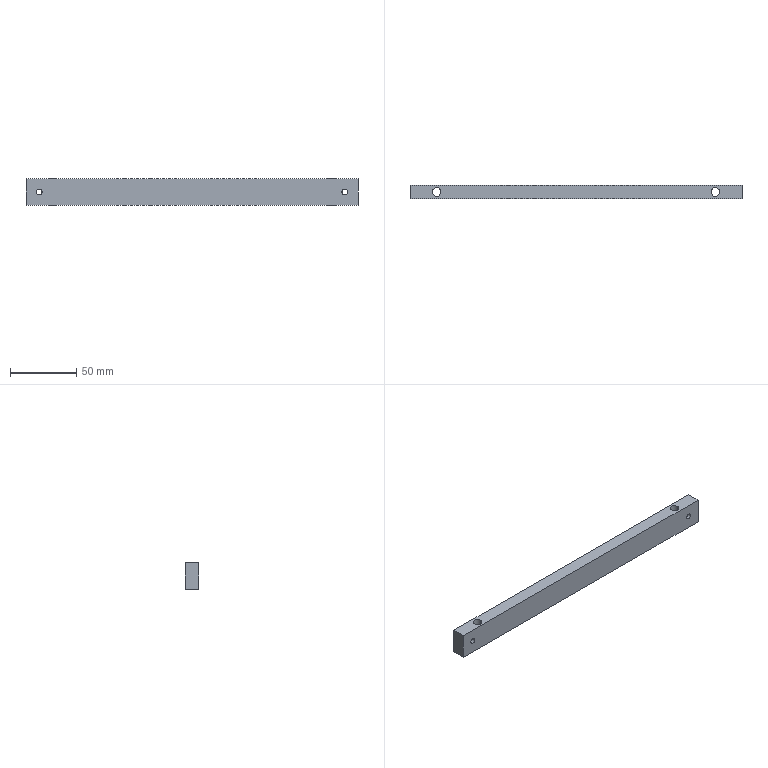Part | STEP file | Insert strip | 1 solid | 14 faces | box 250 x 10 x 20 mm | volume 48396 mm3 | cylinder 8 | plane 6 | commonest cylinder face diameters 4.2 x4 6.5 x4
STEP:
#1=CARTESIAN_POINT('',(115.,-5.,7.9));
#2=VERTEX_POINT('',#1);
#3=CARTESIAN_POINT('',(115.,-5.,12.1));
#4=VERTEX_POINT('',#3);
#5=CARTESIAN_POINT('',(115.,-5.,10.));
#6=DIRECTION('',(0.,1.,0.));
#7=DIRECTION('',(0.,0.,1.));
#8=AXIS2_PLACEMENT_3D('',#5,#6,#7);
#9=CIRCLE('',#8,2.1);
#10=EDGE_CURVE('',#2,#4,#9,.T.);
#11=ORIENTED_EDGE('',*,*,#10,.F.);
#12=CARTESIAN_POINT('',(115.,5.,7.9));
#13=VERTEX_POINT('',#12);
#14=CARTESIAN_POINT('',(115.,5.,7.9));
#15=DIRECTION('',(0.,1.,0.));
#16=VECTOR('',#15,1000.);
#17=LINE('',#14,#16);
#18=EDGE_CURVE('',#2,#13,#17,.T.);
#19=ORIENTED_EDGE('',*,*,#18,.T.);
#20=CARTESIAN_POINT('',(115.,5.,12.1));
#21=VERTEX_POINT('',#20);
#22=CARTESIAN_POINT('',(115.,5.,10.));
#23=DIRECTION('',(0.,1.,0.));
#24=DIRECTION('',(0.,0.,1.));
#25=AXIS2_PLACEMENT_3D('',#22,#23,#24);
#26=CIRCLE('',#25,2.1);
#27=EDGE_CURVE('',#13,#21,#26,.T.);
#28=ORIENTED_EDGE('',*,*,#27,.T.);
#29=CARTESIAN_POINT('',(115.,5.,12.1));
#30=DIRECTION('',(0.,1.,0.));
#31=VECTOR('',#30,1000.);
#32=LINE('',#29,#31);
#33=EDGE_CURVE('',#4,#21,#32,.T.);
#34=ORIENTED_EDGE('',*,*,#33,.F.);
#35=EDGE_LOOP('',(#11,#19,#28,#34));
#36=FACE_OUTER_BOUND('',#35,.T.);
#37=CARTESIAN_POINT('',(115.,5.,10.));
#38=DIRECTION('',(0.,1.,0.));
#39=DIRECTION('',(0.,0.,1.));
#40=AXIS2_PLACEMENT_3D('',#37,#38,#39);
#41=CYLINDRICAL_SURFACE('',#40,2.1);
#42=ADVANCED_FACE('',(#36),#41,.F.);
#43=CARTESIAN_POINT('',(-115.,-5.,7.9));
#44=VERTEX_POINT('',#43);
#45=CARTESIAN_POINT('',(-115.,-5.,12.1));
#46=VERTEX_POINT('',#45);
#47=CARTESIAN_POINT('',(-115.,-5.,10.));
#48=DIRECTION('',(0.,1.,0.));
#49=DIRECTION('',(0.,0.,1.));
#50=AXIS2_PLACEMENT_3D('',#47,#48,#49);
#51=CIRCLE('',#50,2.1);
#52=EDGE_CURVE('',#44,#46,#51,.T.);
#53=ORIENTED_EDGE('',*,*,#52,.F.);
#54=CARTESIAN_POINT('',(-115.,5.,7.9));
#55=VERTEX_POINT('',#54);
#56=CARTESIAN_POINT('',(-115.,5.,7.9));
#57=DIRECTION('',(0.,1.,0.));
#58=VECTOR('',#57,1000.);
#59=LINE('',#56,#58);
#60=EDGE_CURVE('',#44,#55,#59,.T.);
#61=ORIENTED_EDGE('',*,*,#60,.T.);
#62=CARTESIAN_POINT('',(-115.,5.,12.1));
#63=VERTEX_POINT('',#62);
#64=CARTESIAN_POINT('',(-115.,5.,10.));
#65=DIRECTION('',(0.,1.,0.));
#66=DIRECTION('',(0.,0.,1.));
#67=AXIS2_PLACEMENT_3D('',#64,#65,#66);
#68=CIRCLE('',#67,2.1);
#69=EDGE_CURVE('',#55,#63,#68,.T.);
#70=ORIENTED_EDGE('',*,*,#69,.T.);
#71=CARTESIAN_POINT('',(-115.,5.,12.1));
#72=DIRECTION('',(0.,1.,0.));
#73=VECTOR('',#72,1000.);
#74=LINE('',#71,#73);
#75=EDGE_CURVE('',#46,#63,#74,.T.);
#76=ORIENTED_EDGE('',*,*,#75,.F.);
#77=EDGE_LOOP('',(#53,#61,#70,#76));
#78=FACE_OUTER_BOUND('',#77,.T.);
#79=CARTESIAN_POINT('',(-115.,5.,10.));
#80=DIRECTION('',(0.,1.,0.));
#81=DIRECTION('',(0.,0.,1.));
#82=AXIS2_PLACEMENT_3D('',#79,#80,#81);
#83=CYLINDRICAL_SURFACE('',#82,2.1);
#84=ADVANCED_FACE('',(#78),#83,.F.);
#85=CARTESIAN_POINT('',(-108.25,0.,0.));
#86=VERTEX_POINT('',#85);
#87=CARTESIAN_POINT('',(-101.75,0.,0.));
#88=VERTEX_POINT('',#87);
#89=CARTESIAN_POINT('',(-105.,0.,0.));
#90=DIRECTION('',(0.,0.,1.));
#91=DIRECTION('',(1.,0.,0.));
#92=AXIS2_PLACEMENT_3D('',#89,#90,#91);
#93=CIRCLE('',#92,3.25);
#94=EDGE_CURVE('',#86,#88,#93,.T.);
#95=ORIENTED_EDGE('',*,*,#94,.F.);
#96=CARTESIAN_POINT('',(-108.25,0.,20.));
#97=VERTEX_POINT('',#96);
#98=CARTESIAN_POINT('',(-108.25,0.,20.));
#99=DIRECTION('',(0.,0.,1.));
#100=VECTOR('',#99,1000.);
#101=LINE('',#98,#100);
#102=EDGE_CURVE('',#86,#97,#101,.T.);
#103=ORIENTED_EDGE('',*,*,#102,.T.);
#104=CARTESIAN_POINT('',(-101.75,0.,20.));
#105=VERTEX_POINT('',#104);
#106=CARTESIAN_POINT('',(-105.,0.,20.));
#107=DIRECTION('',(0.,0.,1.));
#108=DIRECTION('',(1.,0.,0.));
#109=AXIS2_PLACEMENT_3D('',#106,#107,#108);
#110=CIRCLE('',#109,3.25);
#111=EDGE_CURVE('',#97,#105,#110,.T.);
#112=ORIENTED_EDGE('',*,*,#111,.T.);
#113=CARTESIAN_POINT('',(-101.75,0.,20.));
#114=DIRECTION('',(0.,0.,1.));
#115=VECTOR('',#114,1000.);
#116=LINE('',#113,#115);
#117=EDGE_CURVE('',#88,#105,#116,.T.);
#118=ORIENTED_EDGE('',*,*,#117,.F.);
#119=EDGE_LOOP('',(#95,#103,#112,#118));
#120=FACE_OUTER_BOUND('',#119,.T.);
#121=CARTESIAN_POINT('',(-105.,0.,20.));
#122=DIRECTION('',(0.,0.,1.));
#123=DIRECTION('',(1.,0.,0.));
#124=AXIS2_PLACEMENT_3D('',#121,#122,#123);
#125=CYLINDRICAL_SURFACE('',#124,3.25);
#126=ADVANCED_FACE('',(#120),#125,.F.);
#127=CARTESIAN_POINT('',(101.75,0.,0.));
#128=VERTEX_POINT('',#127);
#129=CARTESIAN_POINT('',(108.25,0.,0.));
#130=VERTEX_POINT('',#129);
#131=CARTESIAN_POINT('',(105.,0.,0.));
#132=DIRECTION('',(0.,0.,1.));
#133=DIRECTION('',(1.,0.,0.));
#134=AXIS2_PLACEMENT_3D('',#131,#132,#133);
#135=CIRCLE('',#134,3.25);
#136=EDGE_CURVE('',#128,#130,#135,.T.);
#137=ORIENTED_EDGE('',*,*,#136,.F.);
#138=CARTESIAN_POINT('',(101.75,0.,20.));
#139=VERTEX_POINT('',#138);
#140=CARTESIAN_POINT('',(101.75,0.,20.));
#141=DIRECTION('',(0.,0.,1.));
#142=VECTOR('',#141,1000.);
#143=LINE('',#140,#142);
#144=EDGE_CURVE('',#128,#139,#143,.T.);
#145=ORIENTED_EDGE('',*,*,#144,.T.);
#146=CARTESIAN_POINT('',(108.25,0.,20.));
#147=VERTEX_POINT('',#146);
#148=CARTESIAN_POINT('',(105.,0.,20.));
#149=DIRECTION('',(0.,0.,1.));
#150=DIRECTION('',(1.,0.,0.));
#151=AXIS2_PLACEMENT_3D('',#148,#149,#150);
#152=CIRCLE('',#151,3.25);
#153=EDGE_CURVE('',#139,#147,#152,.T.);
#154=ORIENTED_EDGE('',*,*,#153,.T.);
#155=CARTESIAN_POINT('',(108.25,0.,20.));
#156=DIRECTION('',(0.,0.,1.));
#157=VECTOR('',#156,1000.);
#158=LINE('',#155,#157);
#159=EDGE_CURVE('',#130,#147,#158,.T.);
#160=ORIENTED_EDGE('',*,*,#159,.F.);
#161=EDGE_LOOP('',(#137,#145,#154,#160));
#162=FACE_OUTER_BOUND('',#161,.T.);
#163=CARTESIAN_POINT('',(105.,0.,20.));
#164=DIRECTION('',(0.,0.,1.));
#165=DIRECTION('',(1.,0.,0.));
#166=AXIS2_PLACEMENT_3D('',#163,#164,#165);
#167=CYLINDRICAL_SURFACE('',#166,3.25);
#168=ADVANCED_FACE('',(#162),#167,.F.);
#169=CARTESIAN_POINT('',(125.,-5.,0.));
#170=VERTEX_POINT('',#169);
#171=CARTESIAN_POINT('',(125.,5.,0.));
#172=VERTEX_POINT('',#171);
#173=CARTESIAN_POINT('',(125.,-5.,0.));
#174=DIRECTION('',(0.,1.,0.));
#175=VECTOR('',#174,1000.);
#176=LINE('',#173,#175);
#177=EDGE_CURVE('',#170,#172,#176,.T.);
#178=ORIENTED_EDGE('',*,*,#177,.T.);
#179=CARTESIAN_POINT('',(125.,5.,20.));
#180=VERTEX_POINT('',#179);
#181=CARTESIAN_POINT('',(125.,5.,20.));
#182=DIRECTION('',(0.,0.,-1.));
#183=VECTOR('',#182,1000.);
#184=LINE('',#181,#183);
#185=EDGE_CURVE('',#180,#172,#184,.T.);
#186=ORIENTED_EDGE('',*,*,#185,.F.);
#187=CARTESIAN_POINT('',(125.,-5.,20.));
#188=VERTEX_POINT('',#187);
#189=CARTESIAN_POINT('',(125.,-5.,20.));
#190=DIRECTION('',(0.,1.,0.));
#191=VECTOR('',#190,1000.);
#192=LINE('',#189,#191);
#193=EDGE_CURVE('',#188,#180,#192,.T.);
#194=ORIENTED_EDGE('',*,*,#193,.F.);
#195=CARTESIAN_POINT('',(125.,-5.,20.));
#196=DIRECTION('',(0.,0.,-1.));
#197=VECTOR('',#196,1000.);
#198=LINE('',#195,#197);
#199=EDGE_CURVE('',#188,#170,#198,.T.);
#200=ORIENTED_EDGE('',*,*,#199,.T.);
#201=EDGE_LOOP('',(#178,#186,#194,#200));
#202=FACE_OUTER_BOUND('',#201,.T.);
#203=CARTESIAN_POINT('',(125.,-5.,20.));
#204=DIRECTION('',(-1.,0.,0.));
#205=DIRECTION('',(0.,0.,1.));
#206=AXIS2_PLACEMENT_3D('',#203,#204,#205);
#207=PLANE('',#206);
#208=ADVANCED_FACE('',(#202),#207,.F.);
#209=CARTESIAN_POINT('',(115.,5.,10.));
#210=DIRECTION('',(0.,1.,0.));
#211=DIRECTION('',(0.,0.,1.));
#212=AXIS2_PLACEMENT_3D('',#209,#210,#211);
#213=CIRCLE('',#212,2.1);
#214=EDGE_CURVE('',#21,#13,#213,.T.);
#215=ORIENTED_EDGE('',*,*,#214,.F.);
#216=ORIENTED_EDGE('',*,*,#27,.F.);
#217=EDGE_LOOP('',(#215,#216));
#218=FACE_BOUND('',#217,.T.);
#219=CARTESIAN_POINT('',(-115.,5.,10.));
#220=DIRECTION('',(0.,1.,0.));
#221=DIRECTION('',(0.,0.,1.));
#222=AXIS2_PLACEMENT_3D('',#219,#220,#221);
#223=CIRCLE('',#222,2.1);
#224=EDGE_CURVE('',#63,#55,#223,.T.);
#225=ORIENTED_EDGE('',*,*,#224,.F.);
#226=ORIENTED_EDGE('',*,*,#69,.F.);
#227=EDGE_LOOP('',(#225,#226));
#228=FACE_BOUND('',#227,.T.);
#229=CARTESIAN_POINT('',(-125.,5.,0.));
#230=VERTEX_POINT('',#229);
#231=CARTESIAN_POINT('',(-125.,5.,0.));
#232=DIRECTION('',(-1.,0.,0.));
#233=VECTOR('',#232,1000.);
#234=LINE('',#231,#233);
#235=EDGE_CURVE('',#172,#230,#234,.T.);
#236=ORIENTED_EDGE('',*,*,#235,.T.);
#237=CARTESIAN_POINT('',(-125.,5.,20.));
#238=VERTEX_POINT('',#237);
#239=CARTESIAN_POINT('',(-125.,5.,20.));
#240=DIRECTION('',(0.,0.,-1.));
#241=VECTOR('',#240,1000.);
#242=LINE('',#239,#241);
#243=EDGE_CURVE('',#238,#230,#242,.T.);
#244=ORIENTED_EDGE('',*,*,#243,.F.);
#245=CARTESIAN_POINT('',(-125.,5.,20.));
#246=DIRECTION('',(-1.,0.,0.));
#247=VECTOR('',#246,1000.);
#248=LINE('',#245,#247);
#249=EDGE_CURVE('',#180,#238,#248,.T.);
#250=ORIENTED_EDGE('',*,*,#249,.F.);
#251=ORIENTED_EDGE('',*,*,#185,.T.);
#252=EDGE_LOOP('',(#236,#244,#250,#251));
#253=FACE_OUTER_BOUND('',#252,.T.);
#254=CARTESIAN_POINT('',(-125.,5.,20.));
#255=DIRECTION('',(0.,-1.,0.));
#256=DIRECTION('',(0.,0.,-1.));
#257=AXIS2_PLACEMENT_3D('',#254,#255,#256);
#258=PLANE('',#257);
#259=ADVANCED_FACE('',(#218,#228,#253),#258,.F.);
#260=CARTESIAN_POINT('',(-125.,-5.,0.));
#261=VERTEX_POINT('',#260);
#262=CARTESIAN_POINT('',(-125.,-5.,0.));
#263=DIRECTION('',(0.,-1.,0.));
#264=VECTOR('',#263,1000.);
#265=LINE('',#262,#264);
#266=EDGE_CURVE('',#230,#261,#265,.T.);
#267=ORIENTED_EDGE('',*,*,#266,.T.);
#268=CARTESIAN_POINT('',(-125.,-5.,20.));
#269=VERTEX_POINT('',#268);
#270=CARTESIAN_POINT('',(-125.,-5.,20.));
#271=DIRECTION('',(0.,0.,-1.));
#272=VECTOR('',#271,1000.);
#273=LINE('',#270,#272);
#274=EDGE_CURVE('',#269,#261,#273,.T.);
#275=ORIENTED_EDGE('',*,*,#274,.F.);
#276=CARTESIAN_POINT('',(-125.,-5.,20.));
#277=DIRECTION('',(0.,-1.,0.));
#278=VECTOR('',#277,1000.);
#279=LINE('',#276,#278);
#280=EDGE_CURVE('',#238,#269,#279,.T.);
#281=ORIENTED_EDGE('',*,*,#280,.F.);
#282=ORIENTED_EDGE('',*,*,#243,.T.);
#283=EDGE_LOOP('',(#267,#275,#281,#282));
#284=FACE_OUTER_BOUND('',#283,.T.);
#285=CARTESIAN_POINT('',(-125.,-5.,20.));
#286=DIRECTION('',(1.,0.,0.));
#287=DIRECTION('',(0.,0.,-1.));
#288=AXIS2_PLACEMENT_3D('',#285,#286,#287);
#289=PLANE('',#288);
#290=ADVANCED_FACE('',(#284),#289,.F.);
#291=CARTESIAN_POINT('',(115.,-5.,10.));
#292=DIRECTION('',(0.,1.,0.));
#293=DIRECTION('',(0.,0.,1.));
#294=AXIS2_PLACEMENT_3D('',#291,#292,#293);
#295=CIRCLE('',#294,2.1);
#296=EDGE_CURVE('',#4,#2,#295,.T.);
#297=ORIENTED_EDGE('',*,*,#296,.T.);
#298=ORIENTED_EDGE('',*,*,#10,.T.);
#299=EDGE_LOOP('',(#297,#298));
#300=FACE_BOUND('',#299,.T.);
#301=CARTESIAN_POINT('',(-115.,-5.,10.));
#302=DIRECTION('',(0.,1.,0.));
#303=DIRECTION('',(0.,0.,1.));
#304=AXIS2_PLACEMENT_3D('',#301,#302,#303);
#305=CIRCLE('',#304,2.1);
#306=EDGE_CURVE('',#46,#44,#305,.T.);
#307=ORIENTED_EDGE('',*,*,#306,.T.);
#308=ORIENTED_EDGE('',*,*,#52,.T.);
#309=EDGE_LOOP('',(#307,#308));
#310=FACE_BOUND('',#309,.T.);
#311=CARTESIAN_POINT('',(-125.,-5.,0.));
#312=DIRECTION('',(1.,0.,0.));
#313=VECTOR('',#312,1000.);
#314=LINE('',#311,#313);
#315=EDGE_CURVE('',#261,#170,#314,.T.);
#316=ORIENTED_EDGE('',*,*,#315,.T.);
#317=ORIENTED_EDGE('',*,*,#199,.F.);
#318=CARTESIAN_POINT('',(-125.,-5.,20.));
#319=DIRECTION('',(1.,0.,0.));
#320=VECTOR('',#319,1000.);
#321=LINE('',#318,#320);
#322=EDGE_CURVE('',#269,#188,#321,.T.);
#323=ORIENTED_EDGE('',*,*,#322,.F.);
#324=ORIENTED_EDGE('',*,*,#274,.T.);
#325=EDGE_LOOP('',(#316,#317,#323,#324));
#326=FACE_OUTER_BOUND('',#325,.T.);
#327=CARTESIAN_POINT('',(-125.,-5.,20.));
#328=DIRECTION('',(0.,1.,0.));
#329=DIRECTION('',(0.,0.,1.));
#330=AXIS2_PLACEMENT_3D('',#327,#328,#329);
#331=PLANE('',#330);
#332=ADVANCED_FACE('',(#300,#310,#326),#331,.F.);
#333=CARTESIAN_POINT('',(-105.,0.,20.));
#334=DIRECTION('',(0.,0.,1.));
#335=DIRECTION('',(1.,0.,0.));
#336=AXIS2_PLACEMENT_3D('',#333,#334,#335);
#337=CIRCLE('',#336,3.25);
#338=EDGE_CURVE('',#105,#97,#337,.T.);
#339=ORIENTED_EDGE('',*,*,#338,.F.);
#340=ORIENTED_EDGE('',*,*,#111,.F.);
#341=EDGE_LOOP('',(#339,#340));
#342=FACE_BOUND('',#341,.T.);
#343=CARTESIAN_POINT('',(105.,0.,20.));
#344=DIRECTION('',(0.,0.,1.));
#345=DIRECTION('',(1.,0.,0.));
#346=AXIS2_PLACEMENT_3D('',#343,#344,#345);
#347=CIRCLE('',#346,3.25);
#348=EDGE_CURVE('',#147,#139,#347,.T.);
#349=ORIENTED_EDGE('',*,*,#348,.F.);
#350=ORIENTED_EDGE('',*,*,#153,.F.);
#351=EDGE_LOOP('',(#349,#350));
#352=FACE_BOUND('',#351,.T.);
#353=ORIENTED_EDGE('',*,*,#193,.T.);
#354=ORIENTED_EDGE('',*,*,#249,.T.);
#355=ORIENTED_EDGE('',*,*,#280,.T.);
#356=ORIENTED_EDGE('',*,*,#322,.T.);
#357=EDGE_LOOP('',(#353,#354,#355,#356));
#358=FACE_OUTER_BOUND('',#357,.T.);
#359=CARTESIAN_POINT('',(125.,5.,20.));
#360=DIRECTION('',(0.,0.,-1.));
#361=DIRECTION('',(-1.,0.,0.));
#362=AXIS2_PLACEMENT_3D('',#359,#360,#361);
#363=PLANE('',#362);
#364=ADVANCED_FACE('',(#342,#352,#358),#363,.F.);
#365=CARTESIAN_POINT('',(-105.,0.,0.));
#366=DIRECTION('',(0.,0.,1.));
#367=DIRECTION('',(1.,0.,0.));
#368=AXIS2_PLACEMENT_3D('',#365,#366,#367);
#369=CIRCLE('',#368,3.25);
#370=EDGE_CURVE('',#88,#86,#369,.T.);
#371=ORIENTED_EDGE('',*,*,#370,.T.);
#372=ORIENTED_EDGE('',*,*,#94,.T.);
#373=EDGE_LOOP('',(#371,#372));
#374=FACE_BOUND('',#373,.T.);
#375=CARTESIAN_POINT('',(105.,0.,0.));
#376=DIRECTION('',(0.,0.,1.));
#377=DIRECTION('',(1.,0.,0.));
#378=AXIS2_PLACEMENT_3D('',#375,#376,#377);
#379=CIRCLE('',#378,3.25);
#380=EDGE_CURVE('',#130,#128,#379,.T.);
#381=ORIENTED_EDGE('',*,*,#380,.T.);
#382=ORIENTED_EDGE('',*,*,#136,.T.);
#383=EDGE_LOOP('',(#381,#382));
#384=FACE_BOUND('',#383,.T.);
#385=ORIENTED_EDGE('',*,*,#177,.F.);
#386=ORIENTED_EDGE('',*,*,#315,.F.);
#387=ORIENTED_EDGE('',*,*,#266,.F.);
#388=ORIENTED_EDGE('',*,*,#235,.F.);
#389=EDGE_LOOP('',(#385,#386,#387,#388));
#390=FACE_OUTER_BOUND('',#389,.T.);
#391=CARTESIAN_POINT('',(125.,5.,0.));
#392=DIRECTION('',(0.,0.,-1.));
#393=DIRECTION('',(-1.,0.,0.));
#394=AXIS2_PLACEMENT_3D('',#391,#392,#393);
#395=PLANE('',#394);
#396=ADVANCED_FACE('',(#374,#384,#390),#395,.T.);
#397=ORIENTED_EDGE('',*,*,#144,.F.);
#398=ORIENTED_EDGE('',*,*,#380,.F.);
#399=ORIENTED_EDGE('',*,*,#159,.T.);
#400=ORIENTED_EDGE('',*,*,#348,.T.);
#401=EDGE_LOOP('',(#397,#398,#399,#400));
#402=FACE_OUTER_BOUND('',#401,.T.);
#403=CARTESIAN_POINT('',(105.,0.,20.));
#404=DIRECTION('',(0.,0.,1.));
#405=DIRECTION('',(1.,0.,0.));
#406=AXIS2_PLACEMENT_3D('',#403,#404,#405);
#407=CYLINDRICAL_SURFACE('',#406,3.25);
#408=ADVANCED_FACE('',(#402),#407,.F.);
#409=ORIENTED_EDGE('',*,*,#102,.F.);
#410=ORIENTED_EDGE('',*,*,#370,.F.);
#411=ORIENTED_EDGE('',*,*,#117,.T.);
#412=ORIENTED_EDGE('',*,*,#338,.T.);
#413=EDGE_LOOP('',(#409,#410,#411,#412));
#414=FACE_OUTER_BOUND('',#413,.T.);
#415=CARTESIAN_POINT('',(-105.,0.,20.));
#416=DIRECTION('',(0.,0.,1.));
#417=DIRECTION('',(1.,0.,0.));
#418=AXIS2_PLACEMENT_3D('',#415,#416,#417);
#419=CYLINDRICAL_SURFACE('',#418,3.25);
#420=ADVANCED_FACE('',(#414),#419,.F.);
#421=ORIENTED_EDGE('',*,*,#60,.F.);
#422=ORIENTED_EDGE('',*,*,#306,.F.);
#423=ORIENTED_EDGE('',*,*,#75,.T.);
#424=ORIENTED_EDGE('',*,*,#224,.T.);
#425=EDGE_LOOP('',(#421,#422,#423,#424));
#426=FACE_OUTER_BOUND('',#425,.T.);
#427=CARTESIAN_POINT('',(-115.,5.,10.));
#428=DIRECTION('',(0.,1.,0.));
#429=DIRECTION('',(0.,0.,1.));
#430=AXIS2_PLACEMENT_3D('',#427,#428,#429);
#431=CYLINDRICAL_SURFACE('',#430,2.1);
#432=ADVANCED_FACE('',(#426),#431,.F.);
#433=ORIENTED_EDGE('',*,*,#18,.F.);
#434=ORIENTED_EDGE('',*,*,#296,.F.);
#435=ORIENTED_EDGE('',*,*,#33,.T.);
#436=ORIENTED_EDGE('',*,*,#214,.T.);
#437=EDGE_LOOP('',(#433,#434,#435,#436));
#438=FACE_OUTER_BOUND('',#437,.T.);
#439=CARTESIAN_POINT('',(115.,5.,10.));
#440=DIRECTION('',(0.,1.,0.));
#441=DIRECTION('',(0.,0.,1.));
#442=AXIS2_PLACEMENT_3D('',#439,#440,#441);
#443=CYLINDRICAL_SURFACE('',#442,2.1);
#444=ADVANCED_FACE('',(#438),#443,.F.);
#445=CLOSED_SHELL('',(#42,#84,#126,#168,#208,#259,#290,#332,#364,#396,#408,#420,#432,#444));
#446=MANIFOLD_SOLID_BREP('',#445);
#447=CARTESIAN_POINT('',(0.,0.,0.));
#448=DIRECTION('',(0.,0.,1.));
#449=DIRECTION('',(1.,0.,0.));
#450=AXIS2_PLACEMENT_3D('',#447,#448,#449);
#451=(LENGTH_UNIT()NAMED_UNIT(*)SI_UNIT(.MILLI.,.METRE.));
#452=UNCERTAINTY_MEASURE_WITH_UNIT(LENGTH_MEASURE(0.00001),#451,'','');
#453=(NAMED_UNIT(*)PLANE_ANGLE_UNIT()SI_UNIT($,.RADIAN.));
#454=(NAMED_UNIT(*)SI_UNIT($,.STERADIAN.)SOLID_ANGLE_UNIT());
#455=(GEOMETRIC_REPRESENTATION_CONTEXT(3)GLOBAL_UNCERTAINTY_ASSIGNED_CONTEXT((#452))GLOBAL_UNIT_ASSIGNED_CONTEXT((#451,#453,#454))REPRESENTATION_CONTEXT('',''));
#456=ADVANCED_BREP_SHAPE_REPRESENTATION('',(#446,#450),#455);